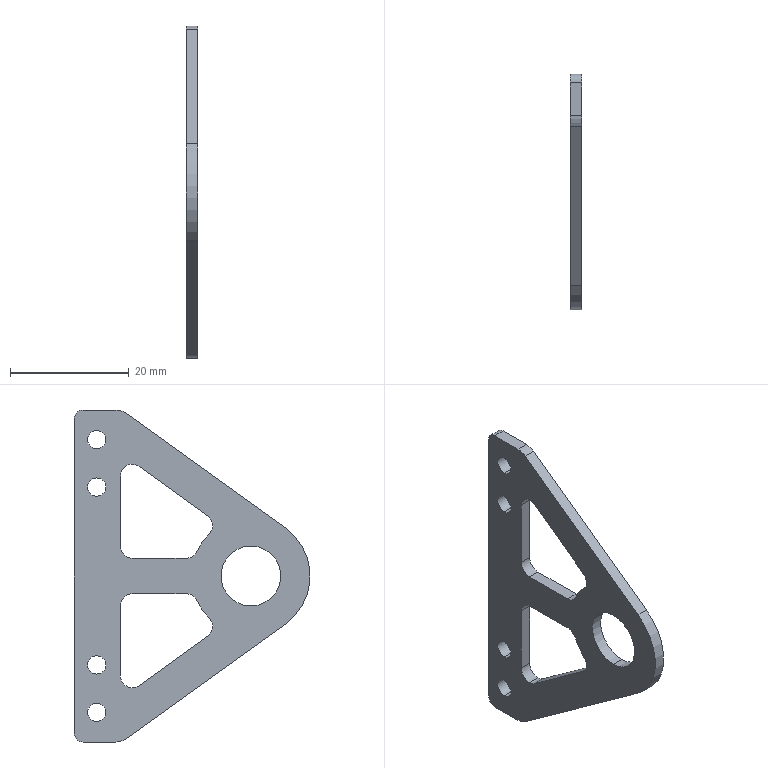Part | SolidWorks | features Fillet 4, Extrusion 1, ICE 1, MirrorPattern 1 | 1 solid | 39 faces | box 2 x 39.8 x 56 mm | volume 2062 mm3 | cylinder 26 | plane 13 | commonest cylinder face diameters 4 x9 3.1 x8 20 x3 3 x2 6 x2 10.1 x2
STEP:
#1=CARTESIAN_POINT('',(0.,20.,-18.85));
#2=VERTEX_POINT('',#1);
#3=CARTESIAN_POINT('',(0.,22.,-16.85));
#4=VERTEX_POINT('',#3);
#5=CARTESIAN_POINT('',(0.,20.,-16.85));
#6=DIRECTION('',(1.,0.,0.));
#7=DIRECTION('',(0.,0.,-1.));
#8=AXIS2_PLACEMENT_3D('',#5,#6,#7);
#9=CIRCLE('',#8,2.);
#10=EDGE_CURVE('',#2,#4,#9,.T.);
#11=ORIENTED_EDGE('',*,*,#10,.F.);
#12=CARTESIAN_POINT('',(2.,20.,-18.85));
#13=VERTEX_POINT('',#12);
#14=CARTESIAN_POINT('',(2.,20.,-18.85));
#15=DIRECTION('',(1.,0.,0.));
#16=VECTOR('',#15,1000.);
#17=LINE('',#14,#16);
#18=EDGE_CURVE('',#2,#13,#17,.T.);
#19=ORIENTED_EDGE('',*,*,#18,.T.);
#20=CARTESIAN_POINT('',(2.,22.,-16.85));
#21=VERTEX_POINT('',#20);
#22=CARTESIAN_POINT('',(2.,20.,-16.85));
#23=DIRECTION('',(-1.,0.,0.));
#24=DIRECTION('',(0.,0.,-1.));
#25=AXIS2_PLACEMENT_3D('',#22,#23,#24);
#26=CIRCLE('',#25,2.);
#27=EDGE_CURVE('',#21,#13,#26,.T.);
#28=ORIENTED_EDGE('',*,*,#27,.F.);
#29=CARTESIAN_POINT('',(2.,22.,-16.85));
#30=DIRECTION('',(1.,0.,0.));
#31=VECTOR('',#30,1000.);
#32=LINE('',#29,#31);
#33=EDGE_CURVE('',#4,#21,#32,.T.);
#34=ORIENTED_EDGE('',*,*,#33,.F.);
#35=EDGE_LOOP('',(#11,#19,#28,#34));
#36=FACE_OUTER_BOUND('',#35,.T.);
#37=CARTESIAN_POINT('',(2.,20.,-16.85));
#38=DIRECTION('',(1.,0.,0.));
#39=DIRECTION('',(0.,0.,-1.));
#40=AXIS2_PLACEMENT_3D('',#37,#38,#39);
#41=CYLINDRICAL_SURFACE('',#40,2.);
#42=ADVANCED_FACE('',(#36),#41,.F.);
#43=CARTESIAN_POINT('',(2.,26.,-13.45));
#44=VERTEX_POINT('',#43);
#45=CARTESIAN_POINT('',(2.,26.,-16.55));
#46=VERTEX_POINT('',#45);
#47=CARTESIAN_POINT('',(2.,26.,-15.));
#48=DIRECTION('',(1.,0.,0.));
#49=DIRECTION('',(0.,0.,1.));
#50=AXIS2_PLACEMENT_3D('',#47,#48,#49);
#51=CIRCLE('',#50,1.55);
#52=EDGE_CURVE('',#44,#46,#51,.T.);
#53=ORIENTED_EDGE('',*,*,#52,.T.);
#54=CARTESIAN_POINT('',(0.,26.,-16.55));
#55=VERTEX_POINT('',#54);
#56=CARTESIAN_POINT('',(2.,26.,-16.55));
#57=DIRECTION('',(-1.,0.,0.));
#58=VECTOR('',#57,1000.);
#59=LINE('',#56,#58);
#60=EDGE_CURVE('',#46,#55,#59,.T.);
#61=ORIENTED_EDGE('',*,*,#60,.T.);
#62=CARTESIAN_POINT('',(0.,26.,-13.45));
#63=VERTEX_POINT('',#62);
#64=CARTESIAN_POINT('',(0.,26.,-15.));
#65=DIRECTION('',(1.,0.,0.));
#66=DIRECTION('',(0.,0.,1.));
#67=AXIS2_PLACEMENT_3D('',#64,#65,#66);
#68=CIRCLE('',#67,1.55);
#69=EDGE_CURVE('',#63,#55,#68,.T.);
#70=ORIENTED_EDGE('',*,*,#69,.F.);
#71=CARTESIAN_POINT('',(2.,26.,-13.45));
#72=DIRECTION('',(-1.,0.,0.));
#73=VECTOR('',#72,1000.);
#74=LINE('',#71,#73);
#75=EDGE_CURVE('',#44,#63,#74,.T.);
#76=ORIENTED_EDGE('',*,*,#75,.F.);
#77=EDGE_LOOP('',(#53,#61,#70,#76));
#78=FACE_OUTER_BOUND('',#77,.T.);
#79=CARTESIAN_POINT('',(2.,26.,-15.));
#80=DIRECTION('',(-1.,0.,0.));
#81=DIRECTION('',(0.,0.,1.));
#82=AXIS2_PLACEMENT_3D('',#79,#80,#81);
#83=CYLINDRICAL_SURFACE('',#82,1.55);
#84=ADVANCED_FACE('',(#78),#83,.F.);
#85=CARTESIAN_POINT('',(2.,26.,-21.45));
#86=VERTEX_POINT('',#85);
#87=CARTESIAN_POINT('',(2.,26.,-24.55));
#88=VERTEX_POINT('',#87);
#89=CARTESIAN_POINT('',(2.,26.,-23.));
#90=DIRECTION('',(1.,0.,0.));
#91=DIRECTION('',(0.,0.,1.));
#92=AXIS2_PLACEMENT_3D('',#89,#90,#91);
#93=CIRCLE('',#92,1.55);
#94=EDGE_CURVE('',#86,#88,#93,.T.);
#95=ORIENTED_EDGE('',*,*,#94,.T.);
#96=CARTESIAN_POINT('',(0.,26.,-24.55));
#97=VERTEX_POINT('',#96);
#98=CARTESIAN_POINT('',(2.,26.,-24.55));
#99=DIRECTION('',(-1.,0.,0.));
#100=VECTOR('',#99,1000.);
#101=LINE('',#98,#100);
#102=EDGE_CURVE('',#88,#97,#101,.T.);
#103=ORIENTED_EDGE('',*,*,#102,.T.);
#104=CARTESIAN_POINT('',(0.,26.,-21.45));
#105=VERTEX_POINT('',#104);
#106=CARTESIAN_POINT('',(0.,26.,-23.));
#107=DIRECTION('',(1.,0.,0.));
#108=DIRECTION('',(0.,0.,1.));
#109=AXIS2_PLACEMENT_3D('',#106,#107,#108);
#110=CIRCLE('',#109,1.55);
#111=EDGE_CURVE('',#105,#97,#110,.T.);
#112=ORIENTED_EDGE('',*,*,#111,.F.);
#113=CARTESIAN_POINT('',(2.,26.,-21.45));
#114=DIRECTION('',(-1.,0.,0.));
#115=VECTOR('',#114,1000.);
#116=LINE('',#113,#115);
#117=EDGE_CURVE('',#86,#105,#116,.T.);
#118=ORIENTED_EDGE('',*,*,#117,.F.);
#119=EDGE_LOOP('',(#95,#103,#112,#118));
#120=FACE_OUTER_BOUND('',#119,.T.);
#121=CARTESIAN_POINT('',(2.,26.,-23.));
#122=DIRECTION('',(-1.,0.,0.));
#123=DIRECTION('',(0.,0.,1.));
#124=AXIS2_PLACEMENT_3D('',#121,#122,#123);
#125=CYLINDRICAL_SURFACE('',#124,1.55);
#126=ADVANCED_FACE('',(#120),#125,.F.);
#127=CARTESIAN_POINT('',(2.,26.,24.55));
#128=VERTEX_POINT('',#127);
#129=CARTESIAN_POINT('',(2.,26.,21.45));
#130=VERTEX_POINT('',#129);
#131=CARTESIAN_POINT('',(2.,26.,23.));
#132=DIRECTION('',(1.,0.,0.));
#133=DIRECTION('',(0.,0.,-1.));
#134=AXIS2_PLACEMENT_3D('',#131,#132,#133);
#135=CIRCLE('',#134,1.55);
#136=EDGE_CURVE('',#128,#130,#135,.T.);
#137=ORIENTED_EDGE('',*,*,#136,.T.);
#138=CARTESIAN_POINT('',(0.,26.,21.45));
#139=VERTEX_POINT('',#138);
#140=CARTESIAN_POINT('',(2.,26.,21.45));
#141=DIRECTION('',(-1.,0.,0.));
#142=VECTOR('',#141,1000.);
#143=LINE('',#140,#142);
#144=EDGE_CURVE('',#130,#139,#143,.T.);
#145=ORIENTED_EDGE('',*,*,#144,.T.);
#146=CARTESIAN_POINT('',(0.,26.,24.55));
#147=VERTEX_POINT('',#146);
#148=CARTESIAN_POINT('',(0.,26.,23.));
#149=DIRECTION('',(1.,0.,0.));
#150=DIRECTION('',(0.,0.,-1.));
#151=AXIS2_PLACEMENT_3D('',#148,#149,#150);
#152=CIRCLE('',#151,1.55);
#153=EDGE_CURVE('',#147,#139,#152,.T.);
#154=ORIENTED_EDGE('',*,*,#153,.F.);
#155=CARTESIAN_POINT('',(2.,26.,24.55));
#156=DIRECTION('',(-1.,0.,0.));
#157=VECTOR('',#156,1000.);
#158=LINE('',#155,#157);
#159=EDGE_CURVE('',#128,#147,#158,.T.);
#160=ORIENTED_EDGE('',*,*,#159,.F.);
#161=EDGE_LOOP('',(#137,#145,#154,#160));
#162=FACE_OUTER_BOUND('',#161,.T.);
#163=CARTESIAN_POINT('',(2.,26.,23.));
#164=DIRECTION('',(-1.,0.,0.));
#165=DIRECTION('',(0.,0.,1.));
#166=AXIS2_PLACEMENT_3D('',#163,#164,#165);
#167=CYLINDRICAL_SURFACE('',#166,1.55);
#168=ADVANCED_FACE('',(#162),#167,.F.);
#169=CARTESIAN_POINT('',(2.,26.,16.55));
#170=VERTEX_POINT('',#169);
#171=CARTESIAN_POINT('',(2.,26.,13.45));
#172=VERTEX_POINT('',#171);
#173=CARTESIAN_POINT('',(2.,26.,15.));
#174=DIRECTION('',(1.,0.,0.));
#175=DIRECTION('',(0.,0.,-1.));
#176=AXIS2_PLACEMENT_3D('',#173,#174,#175);
#177=CIRCLE('',#176,1.55);
#178=EDGE_CURVE('',#170,#172,#177,.T.);
#179=ORIENTED_EDGE('',*,*,#178,.T.);
#180=CARTESIAN_POINT('',(0.,26.,13.45));
#181=VERTEX_POINT('',#180);
#182=CARTESIAN_POINT('',(2.,26.,13.45));
#183=DIRECTION('',(-1.,0.,0.));
#184=VECTOR('',#183,1000.);
#185=LINE('',#182,#184);
#186=EDGE_CURVE('',#172,#181,#185,.T.);
#187=ORIENTED_EDGE('',*,*,#186,.T.);
#188=CARTESIAN_POINT('',(0.,26.,16.55));
#189=VERTEX_POINT('',#188);
#190=CARTESIAN_POINT('',(0.,26.,15.));
#191=DIRECTION('',(1.,0.,0.));
#192=DIRECTION('',(0.,0.,-1.));
#193=AXIS2_PLACEMENT_3D('',#190,#191,#192);
#194=CIRCLE('',#193,1.55);
#195=EDGE_CURVE('',#189,#181,#194,.T.);
#196=ORIENTED_EDGE('',*,*,#195,.F.);
#197=CARTESIAN_POINT('',(2.,26.,16.55));
#198=DIRECTION('',(-1.,0.,0.));
#199=VECTOR('',#198,1000.);
#200=LINE('',#197,#199);
#201=EDGE_CURVE('',#170,#189,#200,.T.);
#202=ORIENTED_EDGE('',*,*,#201,.F.);
#203=EDGE_LOOP('',(#179,#187,#196,#202));
#204=FACE_OUTER_BOUND('',#203,.T.);
#205=CARTESIAN_POINT('',(2.,26.,15.));
#206=DIRECTION('',(-1.,0.,0.));
#207=DIRECTION('',(0.,0.,1.));
#208=AXIS2_PLACEMENT_3D('',#205,#206,#207);
#209=CYLINDRICAL_SURFACE('',#208,1.55);
#210=ADVANCED_FACE('',(#204),#209,.F.);
#211=CARTESIAN_POINT('',(2.,0.,5.05));
#212=VERTEX_POINT('',#211);
#213=CARTESIAN_POINT('',(2.,0.,-5.05));
#214=VERTEX_POINT('',#213);
#215=CARTESIAN_POINT('',(2.,0.,0.));
#216=DIRECTION('',(1.,0.,0.));
#217=DIRECTION('',(0.,0.,-1.));
#218=AXIS2_PLACEMENT_3D('',#215,#216,#217);
#219=CIRCLE('',#218,5.05);
#220=EDGE_CURVE('',#212,#214,#219,.T.);
#221=ORIENTED_EDGE('',*,*,#220,.T.);
#222=CARTESIAN_POINT('',(0.,0.,-5.05));
#223=VERTEX_POINT('',#222);
#224=CARTESIAN_POINT('',(2.,0.,-5.05));
#225=DIRECTION('',(-1.,0.,0.));
#226=VECTOR('',#225,1000.);
#227=LINE('',#224,#226);
#228=EDGE_CURVE('',#214,#223,#227,.T.);
#229=ORIENTED_EDGE('',*,*,#228,.T.);
#230=CARTESIAN_POINT('',(0.,0.,5.05));
#231=VERTEX_POINT('',#230);
#232=CARTESIAN_POINT('',(0.,0.,0.));
#233=DIRECTION('',(1.,0.,0.));
#234=DIRECTION('',(0.,0.,-1.));
#235=AXIS2_PLACEMENT_3D('',#232,#233,#234);
#236=CIRCLE('',#235,5.05);
#237=EDGE_CURVE('',#231,#223,#236,.T.);
#238=ORIENTED_EDGE('',*,*,#237,.F.);
#239=CARTESIAN_POINT('',(2.,0.,5.05));
#240=DIRECTION('',(-1.,0.,0.));
#241=VECTOR('',#240,1000.);
#242=LINE('',#239,#241);
#243=EDGE_CURVE('',#212,#231,#242,.T.);
#244=ORIENTED_EDGE('',*,*,#243,.F.);
#245=EDGE_LOOP('',(#221,#229,#238,#244));
#246=FACE_OUTER_BOUND('',#245,.T.);
#247=CARTESIAN_POINT('',(2.,0.,0.));
#248=DIRECTION('',(-1.,0.,0.));
#249=DIRECTION('',(0.,0.,1.));
#250=AXIS2_PLACEMENT_3D('',#247,#248,#249);
#251=CYLINDRICAL_SURFACE('',#250,5.05);
#252=ADVANCED_FACE('',(#246),#251,.F.);
#253=CARTESIAN_POINT('',(2.,10.909,-3.));
#254=VERTEX_POINT('',#253);
#255=CARTESIAN_POINT('',(2.,20.,-3.));
#256=VERTEX_POINT('',#255);
#257=CARTESIAN_POINT('',(2.,22.,-3.));
#258=DIRECTION('',(0.,1.,0.));
#259=VECTOR('',#258,1000.);
#260=LINE('',#257,#259);
#261=EDGE_CURVE('',#254,#256,#260,.T.);
#262=ORIENTED_EDGE('',*,*,#261,.T.);
#263=CARTESIAN_POINT('',(2.,22.,-5.));
#264=VERTEX_POINT('',#263);
#265=CARTESIAN_POINT('',(2.,20.,-5.));
#266=DIRECTION('',(-1.,0.,0.));
#267=DIRECTION('',(0.,0.,-1.));
#268=AXIS2_PLACEMENT_3D('',#265,#266,#267);
#269=CIRCLE('',#268,2.);
#270=EDGE_CURVE('',#256,#264,#269,.T.);
#271=ORIENTED_EDGE('',*,*,#270,.T.);
#272=CARTESIAN_POINT('',(2.,22.,-20.753));
#273=DIRECTION('',(0.,0.,-1.));
#274=VECTOR('',#273,1000.);
#275=LINE('',#272,#274);
#276=EDGE_CURVE('',#264,#21,#275,.T.);
#277=ORIENTED_EDGE('',*,*,#276,.T.);
#278=ORIENTED_EDGE('',*,*,#27,.T.);
#279=CARTESIAN_POINT('',(2.,18.832,-18.474));
#280=VERTEX_POINT('',#279);
#281=CARTESIAN_POINT('',(2.,20.,-16.85));
#282=DIRECTION('',(-1.,0.,0.));
#283=DIRECTION('',(0.,0.,-1.));
#284=AXIS2_PLACEMENT_3D('',#281,#282,#283);
#285=CIRCLE('',#284,2.);
#286=EDGE_CURVE('',#13,#280,#285,.T.);
#287=ORIENTED_EDGE('',*,*,#286,.T.);
#288=CARTESIAN_POINT('',(2.,7.269,-10.157));
#289=VERTEX_POINT('',#288);
#290=CARTESIAN_POINT('',(2.,22.,-20.753));
#291=DIRECTION('',(0.,-0.8118,0.5839));
#292=VECTOR('',#291,1000.);
#293=LINE('',#290,#292);
#294=EDGE_CURVE('',#280,#289,#293,.T.);
#295=ORIENTED_EDGE('',*,*,#294,.T.);
#296=CARTESIAN_POINT('',(2.,7.031,-7.111));
#297=VERTEX_POINT('',#296);
#298=CARTESIAN_POINT('',(2.,8.437,-8.533));
#299=DIRECTION('',(-1.,0.,0.));
#300=DIRECTION('',(0.,0.,-1.));
#301=AXIS2_PLACEMENT_3D('',#298,#299,#300);
#302=CIRCLE('',#301,2.);
#303=EDGE_CURVE('',#289,#297,#302,.T.);
#304=ORIENTED_EDGE('',*,*,#303,.T.);
#305=CARTESIAN_POINT('',(2.,9.091,-4.167));
#306=VERTEX_POINT('',#305);
#307=CARTESIAN_POINT('',(2.,0.,0.));
#308=DIRECTION('',(1.,0.,0.));
#309=DIRECTION('',(0.,0.,1.));
#310=AXIS2_PLACEMENT_3D('',#307,#308,#309);
#311=CIRCLE('',#310,10.);
#312=EDGE_CURVE('',#297,#306,#311,.T.);
#313=ORIENTED_EDGE('',*,*,#312,.T.);
#314=CARTESIAN_POINT('',(2.,10.909,-5.));
#315=DIRECTION('',(-1.,0.,0.));
#316=DIRECTION('',(0.,0.,-1.));
#317=AXIS2_PLACEMENT_3D('',#314,#315,#316);
#318=CIRCLE('',#317,2.);
#319=EDGE_CURVE('',#306,#254,#318,.T.);
#320=ORIENTED_EDGE('',*,*,#319,.T.);
#321=EDGE_LOOP('',(#262,#271,#277,#278,#287,#295,#304,#313,#320));
#322=FACE_BOUND('',#321,.T.);
#323=ORIENTED_EDGE('',*,*,#94,.F.);
#324=CARTESIAN_POINT('',(2.,26.,-23.));
#325=DIRECTION('',(1.,0.,0.));
#326=DIRECTION('',(0.,0.,1.));
#327=AXIS2_PLACEMENT_3D('',#324,#325,#326);
#328=CIRCLE('',#327,1.55);
#329=EDGE_CURVE('',#88,#86,#328,.T.);
#330=ORIENTED_EDGE('',*,*,#329,.F.);
#331=EDGE_LOOP('',(#323,#330));
#332=FACE_BOUND('',#331,.T.);
#333=ORIENTED_EDGE('',*,*,#178,.F.);
#334=CARTESIAN_POINT('',(2.,26.,15.));
#335=DIRECTION('',(1.,0.,0.));
#336=DIRECTION('',(0.,0.,-1.));
#337=AXIS2_PLACEMENT_3D('',#334,#335,#336);
#338=CIRCLE('',#337,1.55);
#339=EDGE_CURVE('',#172,#170,#338,.T.);
#340=ORIENTED_EDGE('',*,*,#339,.F.);
#341=EDGE_LOOP('',(#333,#340));
#342=FACE_BOUND('',#341,.T.);
#343=CARTESIAN_POINT('',(2.,22.767,-28.));
#344=VERTEX_POINT('',#343);
#345=CARTESIAN_POINT('',(2.,28.3,-28.));
#346=VERTEX_POINT('',#345);
#347=CARTESIAN_POINT('',(2.,29.8,-28.));
#348=DIRECTION('',(0.,1.,0.));
#349=VECTOR('',#348,1000.);
#350=LINE('',#347,#349);
#351=EDGE_CURVE('',#344,#346,#350,.T.);
#352=ORIENTED_EDGE('',*,*,#351,.T.);
#353=CARTESIAN_POINT('',(2.,29.8,-26.5));
#354=VERTEX_POINT('',#353);
#355=CARTESIAN_POINT('',(2.,28.3,-26.5));
#356=DIRECTION('',(1.,0.,0.));
#357=DIRECTION('',(0.,0.,-1.));
#358=AXIS2_PLACEMENT_3D('',#355,#356,#357);
#359=CIRCLE('',#358,1.5);
#360=EDGE_CURVE('',#346,#354,#359,.T.);
#361=ORIENTED_EDGE('',*,*,#360,.T.);
#362=CARTESIAN_POINT('',(2.,29.8,26.5));
#363=VERTEX_POINT('',#362);
#364=CARTESIAN_POINT('',(2.,29.8,-28.));
#365=DIRECTION('',(0.,0.,1.));
#366=VECTOR('',#365,1000.);
#367=LINE('',#364,#366);
#368=EDGE_CURVE('',#354,#363,#367,.T.);
#369=ORIENTED_EDGE('',*,*,#368,.T.);
#370=CARTESIAN_POINT('',(2.,28.3,28.));
#371=VERTEX_POINT('',#370);
#372=CARTESIAN_POINT('',(2.,28.3,26.5));
#373=DIRECTION('',(1.,0.,0.));
#374=DIRECTION('',(0.,0.,-1.));
#375=AXIS2_PLACEMENT_3D('',#372,#373,#374);
#376=CIRCLE('',#375,1.5);
#377=EDGE_CURVE('',#363,#371,#376,.T.);
#378=ORIENTED_EDGE('',*,*,#377,.T.);
#379=CARTESIAN_POINT('',(2.,22.767,28.));
#380=VERTEX_POINT('',#379);
#381=CARTESIAN_POINT('',(2.,29.8,28.));
#382=DIRECTION('',(0.,-1.,0.));
#383=VECTOR('',#382,1000.);
#384=LINE('',#381,#383);
#385=EDGE_CURVE('',#371,#380,#384,.T.);
#386=ORIENTED_EDGE('',*,*,#385,.T.);
#387=CARTESIAN_POINT('',(2.,21.015,27.435));
#388=VERTEX_POINT('',#387);
#389=CARTESIAN_POINT('',(2.,22.767,25.));
#390=DIRECTION('',(1.,0.,0.));
#391=DIRECTION('',(0.,0.,-1.));
#392=AXIS2_PLACEMENT_3D('',#389,#390,#391);
#393=CIRCLE('',#392,3.);
#394=EDGE_CURVE('',#380,#388,#393,.T.);
#395=ORIENTED_EDGE('',*,*,#394,.T.);
#396=CARTESIAN_POINT('',(2.,-5.839,8.118));
#397=VERTEX_POINT('',#396);
#398=CARTESIAN_POINT('',(2.,21.8,28.));
#399=DIRECTION('',(0.,-0.8118,-0.5839));
#400=VECTOR('',#399,1000.);
#401=LINE('',#398,#400);
#402=EDGE_CURVE('',#388,#397,#401,.T.);
#403=ORIENTED_EDGE('',*,*,#402,.T.);
#404=CARTESIAN_POINT('',(2.,-5.839,-8.118));
#405=VERTEX_POINT('',#404);
#406=CARTESIAN_POINT('',(2.,0.,0.));
#407=DIRECTION('',(1.,0.,0.));
#408=DIRECTION('',(0.,0.,-1.));
#409=AXIS2_PLACEMENT_3D('',#406,#407,#408);
#410=CIRCLE('',#409,10.);
#411=EDGE_CURVE('',#397,#405,#410,.T.);
#412=ORIENTED_EDGE('',*,*,#411,.T.);
#413=CARTESIAN_POINT('',(2.,21.015,-27.435));
#414=VERTEX_POINT('',#413);
#415=CARTESIAN_POINT('',(2.,21.8,-28.));
#416=DIRECTION('',(0.,0.8118,-0.5839));
#417=VECTOR('',#416,1000.);
#418=LINE('',#415,#417);
#419=EDGE_CURVE('',#405,#414,#418,.T.);
#420=ORIENTED_EDGE('',*,*,#419,.T.);
#421=CARTESIAN_POINT('',(2.,22.767,-25.));
#422=DIRECTION('',(1.,0.,0.));
#423=DIRECTION('',(0.,0.,-1.));
#424=AXIS2_PLACEMENT_3D('',#421,#422,#423);
#425=CIRCLE('',#424,3.);
#426=EDGE_CURVE('',#414,#344,#425,.T.);
#427=ORIENTED_EDGE('',*,*,#426,.T.);
#428=EDGE_LOOP('',(#352,#361,#369,#378,#386,#395,#403,#412,#420,#427));
#429=FACE_OUTER_BOUND('',#428,.T.);
#430=ORIENTED_EDGE('',*,*,#220,.F.);
#431=CARTESIAN_POINT('',(2.,0.,0.));
#432=DIRECTION('',(1.,0.,0.));
#433=DIRECTION('',(0.,0.,-1.));
#434=AXIS2_PLACEMENT_3D('',#431,#432,#433);
#435=CIRCLE('',#434,5.05);
#436=EDGE_CURVE('',#214,#212,#435,.T.);
#437=ORIENTED_EDGE('',*,*,#436,.F.);
#438=EDGE_LOOP('',(#430,#437));
#439=FACE_BOUND('',#438,.T.);
#440=ORIENTED_EDGE('',*,*,#136,.F.);
#441=CARTESIAN_POINT('',(2.,26.,23.));
#442=DIRECTION('',(1.,0.,0.));
#443=DIRECTION('',(0.,0.,-1.));
#444=AXIS2_PLACEMENT_3D('',#441,#442,#443);
#445=CIRCLE('',#444,1.55);
#446=EDGE_CURVE('',#130,#128,#445,.T.);
#447=ORIENTED_EDGE('',*,*,#446,.F.);
#448=EDGE_LOOP('',(#440,#447));
#449=FACE_BOUND('',#448,.T.);
#450=ORIENTED_EDGE('',*,*,#52,.F.);
#451=CARTESIAN_POINT('',(2.,26.,-15.));
#452=DIRECTION('',(1.,0.,0.));
#453=DIRECTION('',(0.,0.,1.));
#454=AXIS2_PLACEMENT_3D('',#451,#452,#453);
#455=CIRCLE('',#454,1.55);
#456=EDGE_CURVE('',#46,#44,#455,.T.);
#457=ORIENTED_EDGE('',*,*,#456,.F.);
#458=EDGE_LOOP('',(#450,#457));
#459=FACE_BOUND('',#458,.T.);
#460=CARTESIAN_POINT('',(2.,18.832,18.474));
#461=VERTEX_POINT('',#460);
#462=CARTESIAN_POINT('',(2.,7.269,10.157));
#463=VERTEX_POINT('',#462);
#464=CARTESIAN_POINT('',(2.,22.,20.753));
#465=DIRECTION('',(0.,-0.8118,-0.5839));
#466=VECTOR('',#465,1000.);
#467=LINE('',#464,#466);
#468=EDGE_CURVE('',#461,#463,#467,.T.);
#469=ORIENTED_EDGE('',*,*,#468,.F.);
#470=CARTESIAN_POINT('',(2.,22.,16.85));
#471=VERTEX_POINT('',#470);
#472=CARTESIAN_POINT('',(2.,20.,16.85));
#473=DIRECTION('',(-1.,0.,0.));
#474=DIRECTION('',(0.,0.,-1.));
#475=AXIS2_PLACEMENT_3D('',#472,#473,#474);
#476=CIRCLE('',#475,2.);
#477=EDGE_CURVE('',#461,#471,#476,.T.);
#478=ORIENTED_EDGE('',*,*,#477,.T.);
#479=CARTESIAN_POINT('',(2.,22.,5.));
#480=VERTEX_POINT('',#479);
#481=CARTESIAN_POINT('',(2.,22.,20.753));
#482=DIRECTION('',(0.,0.,1.));
#483=VECTOR('',#482,1000.);
#484=LINE('',#481,#483);
#485=EDGE_CURVE('',#480,#471,#484,.T.);
#486=ORIENTED_EDGE('',*,*,#485,.F.);
#487=CARTESIAN_POINT('',(2.,20.,3.));
#488=VERTEX_POINT('',#487);
#489=CARTESIAN_POINT('',(2.,20.,5.));
#490=DIRECTION('',(-1.,0.,0.));
#491=DIRECTION('',(0.,0.,-1.));
#492=AXIS2_PLACEMENT_3D('',#489,#490,#491);
#493=CIRCLE('',#492,2.);
#494=EDGE_CURVE('',#480,#488,#493,.T.);
#495=ORIENTED_EDGE('',*,*,#494,.T.);
#496=CARTESIAN_POINT('',(2.,10.909,3.));
#497=VERTEX_POINT('',#496);
#498=CARTESIAN_POINT('',(2.,22.,3.));
#499=DIRECTION('',(0.,1.,0.));
#500=VECTOR('',#499,1000.);
#501=LINE('',#498,#500);
#502=EDGE_CURVE('',#497,#488,#501,.T.);
#503=ORIENTED_EDGE('',*,*,#502,.F.);
#504=CARTESIAN_POINT('',(2.,9.091,4.167));
#505=VERTEX_POINT('',#504);
#506=CARTESIAN_POINT('',(2.,10.909,5.));
#507=DIRECTION('',(-1.,0.,0.));
#508=DIRECTION('',(0.,0.,-1.));
#509=AXIS2_PLACEMENT_3D('',#506,#507,#508);
#510=CIRCLE('',#509,2.);
#511=EDGE_CURVE('',#497,#505,#510,.T.);
#512=ORIENTED_EDGE('',*,*,#511,.T.);
#513=CARTESIAN_POINT('',(2.,7.031,7.111));
#514=VERTEX_POINT('',#513);
#515=CARTESIAN_POINT('',(2.,0.,0.));
#516=DIRECTION('',(-1.,0.,0.));
#517=DIRECTION('',(0.,0.,-1.));
#518=AXIS2_PLACEMENT_3D('',#515,#516,#517);
#519=CIRCLE('',#518,10.);
#520=EDGE_CURVE('',#514,#505,#519,.T.);
#521=ORIENTED_EDGE('',*,*,#520,.F.);
#522=CARTESIAN_POINT('',(2.,8.437,8.533));
#523=DIRECTION('',(-1.,0.,0.));
#524=DIRECTION('',(0.,0.,-1.));
#525=AXIS2_PLACEMENT_3D('',#522,#523,#524);
#526=CIRCLE('',#525,2.);
#527=EDGE_CURVE('',#514,#463,#526,.T.);
#528=ORIENTED_EDGE('',*,*,#527,.T.);
#529=EDGE_LOOP('',(#469,#478,#486,#495,#503,#512,#521,#528));
#530=FACE_BOUND('',#529,.T.);
#531=CARTESIAN_POINT('',(2.,0.,0.));
#532=DIRECTION('',(1.,0.,0.));
#533=DIRECTION('',(0.,0.,-1.));
#534=AXIS2_PLACEMENT_3D('',#531,#532,#533);
#535=PLANE('',#534);
#536=ADVANCED_FACE('',(#322,#332,#342,#429,#439,#449,#459,#530),#535,.T.);
#537=CARTESIAN_POINT('',(0.,18.832,-18.474));
#538=VERTEX_POINT('',#537);
#539=CARTESIAN_POINT('',(0.,7.269,-10.157));
#540=VERTEX_POINT('',#539);
#541=CARTESIAN_POINT('',(0.,22.,-20.753));
#542=DIRECTION('',(0.,-0.8118,0.5839));
#543=VECTOR('',#542,1000.);
#544=LINE('',#541,#543);
#545=EDGE_CURVE('',#538,#540,#544,.T.);
#546=ORIENTED_EDGE('',*,*,#545,.F.);
#547=CARTESIAN_POINT('',(0.,20.,-16.85));
#548=DIRECTION('',(1.,0.,0.));
#549=DIRECTION('',(0.,0.,-1.));
#550=AXIS2_PLACEMENT_3D('',#547,#548,#549);
#551=CIRCLE('',#550,2.);
#552=EDGE_CURVE('',#538,#2,#551,.T.);
#553=ORIENTED_EDGE('',*,*,#552,.T.);
#554=ORIENTED_EDGE('',*,*,#10,.T.);
#555=CARTESIAN_POINT('',(0.,22.,-5.));
#556=VERTEX_POINT('',#555);
#557=CARTESIAN_POINT('',(0.,22.,-20.753));
#558=DIRECTION('',(0.,0.,-1.));
#559=VECTOR('',#558,1000.);
#560=LINE('',#557,#559);
#561=EDGE_CURVE('',#556,#4,#560,.T.);
#562=ORIENTED_EDGE('',*,*,#561,.F.);
#563=CARTESIAN_POINT('',(0.,20.,-3.));
#564=VERTEX_POINT('',#563);
#565=CARTESIAN_POINT('',(0.,20.,-5.));
#566=DIRECTION('',(1.,0.,0.));
#567=DIRECTION('',(0.,0.,-1.));
#568=AXIS2_PLACEMENT_3D('',#565,#566,#567);
#569=CIRCLE('',#568,2.);
#570=EDGE_CURVE('',#556,#564,#569,.T.);
#571=ORIENTED_EDGE('',*,*,#570,.T.);
#572=CARTESIAN_POINT('',(0.,10.909,-3.));
#573=VERTEX_POINT('',#572);
#574=CARTESIAN_POINT('',(0.,22.,-3.));
#575=DIRECTION('',(0.,1.,0.));
#576=VECTOR('',#575,1000.);
#577=LINE('',#574,#576);
#578=EDGE_CURVE('',#573,#564,#577,.T.);
#579=ORIENTED_EDGE('',*,*,#578,.F.);
#580=CARTESIAN_POINT('',(0.,9.091,-4.167));
#581=VERTEX_POINT('',#580);
#582=CARTESIAN_POINT('',(0.,10.909,-5.));
#583=DIRECTION('',(1.,0.,0.));
#584=DIRECTION('',(0.,0.,-1.));
#585=AXIS2_PLACEMENT_3D('',#582,#583,#584);
#586=CIRCLE('',#585,2.);
#587=EDGE_CURVE('',#573,#581,#586,.T.);
#588=ORIENTED_EDGE('',*,*,#587,.T.);
#589=CARTESIAN_POINT('',(0.,7.031,-7.111));
#590=VERTEX_POINT('',#589);
#591=CARTESIAN_POINT('',(0.,0.,0.));
#592=DIRECTION('',(1.,0.,0.));
#593=DIRECTION('',(0.,0.,1.));
#594=AXIS2_PLACEMENT_3D('',#591,#592,#593);
#595=CIRCLE('',#594,10.);
#596=EDGE_CURVE('',#590,#581,#595,.T.);
#597=ORIENTED_EDGE('',*,*,#596,.F.);
#598=CARTESIAN_POINT('',(0.,8.437,-8.533));
#599=DIRECTION('',(1.,0.,0.));
#600=DIRECTION('',(0.,0.,-1.));
#601=AXIS2_PLACEMENT_3D('',#598,#599,#600);
#602=CIRCLE('',#601,2.);
#603=EDGE_CURVE('',#590,#540,#602,.T.);
#604=ORIENTED_EDGE('',*,*,#603,.T.);
#605=EDGE_LOOP('',(#546,#553,#554,#562,#571,#579,#588,#597,#604));
#606=FACE_BOUND('',#605,.T.);
#607=ORIENTED_EDGE('',*,*,#69,.T.);
#608=CARTESIAN_POINT('',(0.,26.,-15.));
#609=DIRECTION('',(1.,0.,0.));
#610=DIRECTION('',(0.,0.,1.));
#611=AXIS2_PLACEMENT_3D('',#608,#609,#610);
#612=CIRCLE('',#611,1.55);
#613=EDGE_CURVE('',#55,#63,#612,.T.);
#614=ORIENTED_EDGE('',*,*,#613,.T.);
#615=EDGE_LOOP('',(#607,#614));
#616=FACE_BOUND('',#615,.T.);
#617=ORIENTED_EDGE('',*,*,#111,.T.);
#618=CARTESIAN_POINT('',(0.,26.,-23.));
#619=DIRECTION('',(1.,0.,0.));
#620=DIRECTION('',(0.,0.,1.));
#621=AXIS2_PLACEMENT_3D('',#618,#619,#620);
#622=CIRCLE('',#621,1.55);
#623=EDGE_CURVE('',#97,#105,#622,.T.);
#624=ORIENTED_EDGE('',*,*,#623,.T.);
#625=EDGE_LOOP('',(#617,#624));
#626=FACE_BOUND('',#625,.T.);
#627=ORIENTED_EDGE('',*,*,#153,.T.);
#628=CARTESIAN_POINT('',(0.,26.,23.));
#629=DIRECTION('',(1.,0.,0.));
#630=DIRECTION('',(0.,0.,-1.));
#631=AXIS2_PLACEMENT_3D('',#628,#629,#630);
#632=CIRCLE('',#631,1.55);
#633=EDGE_CURVE('',#139,#147,#632,.T.);
#634=ORIENTED_EDGE('',*,*,#633,.T.);
#635=EDGE_LOOP('',(#627,#634));
#636=FACE_BOUND('',#635,.T.);
#637=ORIENTED_EDGE('',*,*,#195,.T.);
#638=CARTESIAN_POINT('',(0.,26.,15.));
#639=DIRECTION('',(1.,0.,0.));
#640=DIRECTION('',(0.,0.,-1.));
#641=AXIS2_PLACEMENT_3D('',#638,#639,#640);
#642=CIRCLE('',#641,1.55);
#643=EDGE_CURVE('',#181,#189,#642,.T.);
#644=ORIENTED_EDGE('',*,*,#643,.T.);
#645=EDGE_LOOP('',(#637,#644));
#646=FACE_BOUND('',#645,.T.);
#647=ORIENTED_EDGE('',*,*,#237,.T.);
#648=CARTESIAN_POINT('',(0.,0.,0.));
#649=DIRECTION('',(1.,0.,0.));
#650=DIRECTION('',(0.,0.,-1.));
#651=AXIS2_PLACEMENT_3D('',#648,#649,#650);
#652=CIRCLE('',#651,5.05);
#653=EDGE_CURVE('',#223,#231,#652,.T.);
#654=ORIENTED_EDGE('',*,*,#653,.T.);
#655=EDGE_LOOP('',(#647,#654));
#656=FACE_BOUND('',#655,.T.);
#657=CARTESIAN_POINT('',(0.,29.8,-26.5));
#658=VERTEX_POINT('',#657);
#659=CARTESIAN_POINT('',(0.,29.8,26.5));
#660=VERTEX_POINT('',#659);
#661=CARTESIAN_POINT('',(0.,29.8,-28.));
#662=DIRECTION('',(0.,0.,1.));
#663=VECTOR('',#662,1000.);
#664=LINE('',#661,#663);
#665=EDGE_CURVE('',#658,#660,#664,.T.);
#666=ORIENTED_EDGE('',*,*,#665,.F.);
#667=CARTESIAN_POINT('',(0.,28.3,-28.));
#668=VERTEX_POINT('',#667);
#669=CARTESIAN_POINT('',(0.,28.3,-26.5));
#670=DIRECTION('',(-1.,0.,0.));
#671=DIRECTION('',(0.,0.,-1.));
#672=AXIS2_PLACEMENT_3D('',#669,#670,#671);
#673=CIRCLE('',#672,1.5);
#674=EDGE_CURVE('',#658,#668,#673,.T.);
#675=ORIENTED_EDGE('',*,*,#674,.T.);
#676=CARTESIAN_POINT('',(0.,22.767,-28.));
#677=VERTEX_POINT('',#676);
#678=CARTESIAN_POINT('',(0.,29.8,-28.));
#679=DIRECTION('',(0.,1.,0.));
#680=VECTOR('',#679,1000.);
#681=LINE('',#678,#680);
#682=EDGE_CURVE('',#677,#668,#681,.T.);
#683=ORIENTED_EDGE('',*,*,#682,.F.);
#684=CARTESIAN_POINT('',(0.,21.015,-27.435));
#685=VERTEX_POINT('',#684);
#686=CARTESIAN_POINT('',(0.,22.767,-25.));
#687=DIRECTION('',(-1.,0.,0.));
#688=DIRECTION('',(0.,0.,-1.));
#689=AXIS2_PLACEMENT_3D('',#686,#687,#688);
#690=CIRCLE('',#689,3.);
#691=EDGE_CURVE('',#677,#685,#690,.T.);
#692=ORIENTED_EDGE('',*,*,#691,.T.);
#693=CARTESIAN_POINT('',(0.,-5.839,-8.118));
#694=VERTEX_POINT('',#693);
#695=CARTESIAN_POINT('',(0.,21.8,-28.));
#696=DIRECTION('',(0.,0.8118,-0.5839));
#697=VECTOR('',#696,1000.);
#698=LINE('',#695,#697);
#699=EDGE_CURVE('',#694,#685,#698,.T.);
#700=ORIENTED_EDGE('',*,*,#699,.F.);
#701=CARTESIAN_POINT('',(0.,-5.839,8.118));
#702=VERTEX_POINT('',#701);
#703=CARTESIAN_POINT('',(0.,0.,0.));
#704=DIRECTION('',(1.,0.,0.));
#705=DIRECTION('',(0.,0.,-1.));
#706=AXIS2_PLACEMENT_3D('',#703,#704,#705);
#707=CIRCLE('',#706,10.);
#708=EDGE_CURVE('',#702,#694,#707,.T.);
#709=ORIENTED_EDGE('',*,*,#708,.F.);
#710=CARTESIAN_POINT('',(0.,21.015,27.435));
#711=VERTEX_POINT('',#710);
#712=CARTESIAN_POINT('',(0.,21.8,28.));
#713=DIRECTION('',(0.,-0.8118,-0.5839));
#714=VECTOR('',#713,1000.);
#715=LINE('',#712,#714);
#716=EDGE_CURVE('',#711,#702,#715,.T.);
#717=ORIENTED_EDGE('',*,*,#716,.F.);
#718=CARTESIAN_POINT('',(0.,22.767,28.));
#719=VERTEX_POINT('',#718);
#720=CARTESIAN_POINT('',(0.,22.767,25.));
#721=DIRECTION('',(-1.,0.,0.));
#722=DIRECTION('',(0.,0.,-1.));
#723=AXIS2_PLACEMENT_3D('',#720,#721,#722);
#724=CIRCLE('',#723,3.);
#725=EDGE_CURVE('',#711,#719,#724,.T.);
#726=ORIENTED_EDGE('',*,*,#725,.T.);
#727=CARTESIAN_POINT('',(0.,28.3,28.));
#728=VERTEX_POINT('',#727);
#729=CARTESIAN_POINT('',(0.,29.8,28.));
#730=DIRECTION('',(0.,-1.,0.));
#731=VECTOR('',#730,1000.);
#732=LINE('',#729,#731);
#733=EDGE_CURVE('',#728,#719,#732,.T.);
#734=ORIENTED_EDGE('',*,*,#733,.F.);
#735=CARTESIAN_POINT('',(0.,28.3,26.5));
#736=DIRECTION('',(-1.,0.,0.));
#737=DIRECTION('',(0.,0.,-1.));
#738=AXIS2_PLACEMENT_3D('',#735,#736,#737);
#739=CIRCLE('',#738,1.5);
#740=EDGE_CURVE('',#728,#660,#739,.T.);
#741=ORIENTED_EDGE('',*,*,#740,.T.);
#742=EDGE_LOOP('',(#666,#675,#683,#692,#700,#709,#717,#726,#734,#741));
#743=FACE_OUTER_BOUND('',#742,.T.);
#744=CARTESIAN_POINT('',(0.,10.909,3.));
#745=VERTEX_POINT('',#744);
#746=CARTESIAN_POINT('',(0.,20.,3.));
#747=VERTEX_POINT('',#746);
#748=CARTESIAN_POINT('',(0.,22.,3.));
#749=DIRECTION('',(0.,1.,0.));
#750=VECTOR('',#749,1000.);
#751=LINE('',#748,#750);
#752=EDGE_CURVE('',#745,#747,#751,.T.);
#753=ORIENTED_EDGE('',*,*,#752,.T.);
#754=CARTESIAN_POINT('',(0.,22.,5.));
#755=VERTEX_POINT('',#754);
#756=CARTESIAN_POINT('',(0.,20.,5.));
#757=DIRECTION('',(1.,0.,0.));
#758=DIRECTION('',(0.,0.,-1.));
#759=AXIS2_PLACEMENT_3D('',#756,#757,#758);
#760=CIRCLE('',#759,2.);
#761=EDGE_CURVE('',#747,#755,#760,.T.);
#762=ORIENTED_EDGE('',*,*,#761,.T.);
#763=CARTESIAN_POINT('',(0.,22.,16.85));
#764=VERTEX_POINT('',#763);
#765=CARTESIAN_POINT('',(0.,22.,20.753));
#766=DIRECTION('',(0.,0.,1.));
#767=VECTOR('',#766,1000.);
#768=LINE('',#765,#767);
#769=EDGE_CURVE('',#755,#764,#768,.T.);
#770=ORIENTED_EDGE('',*,*,#769,.T.);
#771=CARTESIAN_POINT('',(0.,18.832,18.474));
#772=VERTEX_POINT('',#771);
#773=CARTESIAN_POINT('',(0.,20.,16.85));
#774=DIRECTION('',(1.,0.,0.));
#775=DIRECTION('',(0.,0.,-1.));
#776=AXIS2_PLACEMENT_3D('',#773,#774,#775);
#777=CIRCLE('',#776,2.);
#778=EDGE_CURVE('',#764,#772,#777,.T.);
#779=ORIENTED_EDGE('',*,*,#778,.T.);
#780=CARTESIAN_POINT('',(0.,7.269,10.157));
#781=VERTEX_POINT('',#780);
#782=CARTESIAN_POINT('',(0.,22.,20.753));
#783=DIRECTION('',(0.,-0.8118,-0.5839));
#784=VECTOR('',#783,1000.);
#785=LINE('',#782,#784);
#786=EDGE_CURVE('',#772,#781,#785,.T.);
#787=ORIENTED_EDGE('',*,*,#786,.T.);
#788=CARTESIAN_POINT('',(0.,7.031,7.111));
#789=VERTEX_POINT('',#788);
#790=CARTESIAN_POINT('',(0.,8.437,8.533));
#791=DIRECTION('',(1.,0.,0.));
#792=DIRECTION('',(0.,0.,-1.));
#793=AXIS2_PLACEMENT_3D('',#790,#791,#792);
#794=CIRCLE('',#793,2.);
#795=EDGE_CURVE('',#781,#789,#794,.T.);
#796=ORIENTED_EDGE('',*,*,#795,.T.);
#797=CARTESIAN_POINT('',(0.,9.091,4.167));
#798=VERTEX_POINT('',#797);
#799=CARTESIAN_POINT('',(0.,0.,0.));
#800=DIRECTION('',(-1.,0.,0.));
#801=DIRECTION('',(0.,0.,-1.));
#802=AXIS2_PLACEMENT_3D('',#799,#800,#801);
#803=CIRCLE('',#802,10.);
#804=EDGE_CURVE('',#789,#798,#803,.T.);
#805=ORIENTED_EDGE('',*,*,#804,.T.);
#806=CARTESIAN_POINT('',(0.,10.909,5.));
#807=DIRECTION('',(1.,0.,0.));
#808=DIRECTION('',(0.,0.,-1.));
#809=AXIS2_PLACEMENT_3D('',#806,#807,#808);
#810=CIRCLE('',#809,2.);
#811=EDGE_CURVE('',#798,#745,#810,.T.);
#812=ORIENTED_EDGE('',*,*,#811,.T.);
#813=EDGE_LOOP('',(#753,#762,#770,#779,#787,#796,#805,#812));
#814=FACE_BOUND('',#813,.T.);
#815=CARTESIAN_POINT('',(0.,0.,0.));
#816=DIRECTION('',(1.,0.,0.));
#817=DIRECTION('',(0.,0.,-1.));
#818=AXIS2_PLACEMENT_3D('',#815,#816,#817);
#819=PLANE('',#818);
#820=ADVANCED_FACE('',(#606,#616,#626,#636,#646,#656,#743,#814),#819,.F.);
#821=ORIENTED_EDGE('',*,*,#368,.F.);
#822=CARTESIAN_POINT('',(2.,29.8,-26.5));
#823=DIRECTION('',(-1.,0.,0.));
#824=VECTOR('',#823,1000.);
#825=LINE('',#822,#824);
#826=EDGE_CURVE('',#354,#658,#825,.T.);
#827=ORIENTED_EDGE('',*,*,#826,.T.);
#828=ORIENTED_EDGE('',*,*,#665,.T.);
#829=CARTESIAN_POINT('',(2.,29.8,26.5));
#830=DIRECTION('',(1.,0.,0.));
#831=VECTOR('',#830,1000.);
#832=LINE('',#829,#831);
#833=EDGE_CURVE('',#660,#363,#832,.T.);
#834=ORIENTED_EDGE('',*,*,#833,.T.);
#835=EDGE_LOOP('',(#821,#827,#828,#834));
#836=FACE_OUTER_BOUND('',#835,.T.);
#837=CARTESIAN_POINT('',(2.,29.8,-28.));
#838=DIRECTION('',(0.,-1.,0.));
#839=DIRECTION('',(0.,0.,-1.));
#840=AXIS2_PLACEMENT_3D('',#837,#838,#839);
#841=PLANE('',#840);
#842=ADVANCED_FACE('',(#836),#841,.F.);
#843=ORIENTED_EDGE('',*,*,#385,.F.);
#844=CARTESIAN_POINT('',(2.,28.3,28.));
#845=DIRECTION('',(-1.,0.,0.));
#846=VECTOR('',#845,1000.);
#847=LINE('',#844,#846);
#848=EDGE_CURVE('',#371,#728,#847,.T.);
#849=ORIENTED_EDGE('',*,*,#848,.T.);
#850=ORIENTED_EDGE('',*,*,#733,.T.);
#851=CARTESIAN_POINT('',(2.,22.767,28.));
#852=DIRECTION('',(1.,0.,0.));
#853=VECTOR('',#852,1000.);
#854=LINE('',#851,#853);
#855=EDGE_CURVE('',#719,#380,#854,.T.);
#856=ORIENTED_EDGE('',*,*,#855,.T.);
#857=EDGE_LOOP('',(#843,#849,#850,#856));
#858=FACE_OUTER_BOUND('',#857,.T.);
#859=CARTESIAN_POINT('',(2.,29.8,28.));
#860=DIRECTION('',(0.,0.,-1.));
#861=DIRECTION('',(0.,1.,0.));
#862=AXIS2_PLACEMENT_3D('',#859,#860,#861);
#863=PLANE('',#862);
#864=ADVANCED_FACE('',(#858),#863,.F.);
#865=ORIENTED_EDGE('',*,*,#402,.F.);
#866=CARTESIAN_POINT('',(2.,21.015,27.435));
#867=DIRECTION('',(-1.,0.,0.));
#868=VECTOR('',#867,1000.);
#869=LINE('',#866,#868);
#870=EDGE_CURVE('',#388,#711,#869,.T.);
#871=ORIENTED_EDGE('',*,*,#870,.T.);
#872=ORIENTED_EDGE('',*,*,#716,.T.);
#873=CARTESIAN_POINT('',(2.,-5.839,8.118));
#874=DIRECTION('',(-1.,0.,0.));
#875=VECTOR('',#874,1000.);
#876=LINE('',#873,#875);
#877=EDGE_CURVE('',#397,#702,#876,.T.);
#878=ORIENTED_EDGE('',*,*,#877,.F.);
#879=EDGE_LOOP('',(#865,#871,#872,#878));
#880=FACE_OUTER_BOUND('',#879,.T.);
#881=CARTESIAN_POINT('',(2.,21.8,28.));
#882=DIRECTION('',(0.,0.5839,-0.8118));
#883=DIRECTION('',(0.,0.8118,0.5839));
#884=AXIS2_PLACEMENT_3D('',#881,#882,#883);
#885=PLANE('',#884);
#886=ADVANCED_FACE('',(#880),#885,.F.);
#887=ORIENTED_EDGE('',*,*,#708,.T.);
#888=CARTESIAN_POINT('',(2.,-5.839,-8.118));
#889=DIRECTION('',(-1.,0.,0.));
#890=VECTOR('',#889,1000.);
#891=LINE('',#888,#890);
#892=EDGE_CURVE('',#405,#694,#891,.T.);
#893=ORIENTED_EDGE('',*,*,#892,.F.);
#894=ORIENTED_EDGE('',*,*,#411,.F.);
#895=ORIENTED_EDGE('',*,*,#877,.T.);
#896=EDGE_LOOP('',(#887,#893,#894,#895));
#897=FACE_OUTER_BOUND('',#896,.T.);
#898=CARTESIAN_POINT('',(2.,0.,0.));
#899=DIRECTION('',(-1.,0.,0.));
#900=DIRECTION('',(0.,0.,1.));
#901=AXIS2_PLACEMENT_3D('',#898,#899,#900);
#902=CYLINDRICAL_SURFACE('',#901,10.);
#903=ADVANCED_FACE('',(#897),#902,.T.);
#904=ORIENTED_EDGE('',*,*,#699,.T.);
#905=CARTESIAN_POINT('',(2.,21.015,-27.435));
#906=DIRECTION('',(1.,0.,0.));
#907=VECTOR('',#906,1000.);
#908=LINE('',#905,#907);
#909=EDGE_CURVE('',#685,#414,#908,.T.);
#910=ORIENTED_EDGE('',*,*,#909,.T.);
#911=ORIENTED_EDGE('',*,*,#419,.F.);
#912=ORIENTED_EDGE('',*,*,#892,.T.);
#913=EDGE_LOOP('',(#904,#910,#911,#912));
#914=FACE_OUTER_BOUND('',#913,.T.);
#915=CARTESIAN_POINT('',(2.,21.8,-28.));
#916=DIRECTION('',(0.,0.5839,0.8118));
#917=DIRECTION('',(0.,-0.8118,0.5839));
#918=AXIS2_PLACEMENT_3D('',#915,#916,#917);
#919=PLANE('',#918);
#920=ADVANCED_FACE('',(#914),#919,.F.);
#921=ORIENTED_EDGE('',*,*,#682,.T.);
#922=CARTESIAN_POINT('',(2.,28.3,-28.));
#923=DIRECTION('',(1.,0.,0.));
#924=VECTOR('',#923,1000.);
#925=LINE('',#922,#924);
#926=EDGE_CURVE('',#668,#346,#925,.T.);
#927=ORIENTED_EDGE('',*,*,#926,.T.);
#928=ORIENTED_EDGE('',*,*,#351,.F.);
#929=CARTESIAN_POINT('',(2.,22.767,-28.));
#930=DIRECTION('',(-1.,0.,0.));
#931=VECTOR('',#930,1000.);
#932=LINE('',#929,#931);
#933=EDGE_CURVE('',#344,#677,#932,.T.);
#934=ORIENTED_EDGE('',*,*,#933,.T.);
#935=EDGE_LOOP('',(#921,#927,#928,#934));
#936=FACE_OUTER_BOUND('',#935,.T.);
#937=CARTESIAN_POINT('',(2.,29.8,-28.));
#938=DIRECTION('',(0.,0.,1.));
#939=DIRECTION('',(0.,-1.,0.));
#940=AXIS2_PLACEMENT_3D('',#937,#938,#939);
#941=PLANE('',#940);
#942=ADVANCED_FACE('',(#936),#941,.F.);
#943=ORIENTED_EDGE('',*,*,#228,.F.);
#944=ORIENTED_EDGE('',*,*,#436,.T.);
#945=ORIENTED_EDGE('',*,*,#243,.T.);
#946=ORIENTED_EDGE('',*,*,#653,.F.);
#947=EDGE_LOOP('',(#943,#944,#945,#946));
#948=FACE_OUTER_BOUND('',#947,.T.);
#949=CARTESIAN_POINT('',(2.,0.,0.));
#950=DIRECTION('',(-1.,0.,0.));
#951=DIRECTION('',(0.,0.,1.));
#952=AXIS2_PLACEMENT_3D('',#949,#950,#951);
#953=CYLINDRICAL_SURFACE('',#952,5.05);
#954=ADVANCED_FACE('',(#948),#953,.F.);
#955=ORIENTED_EDGE('',*,*,#186,.F.);
#956=ORIENTED_EDGE('',*,*,#339,.T.);
#957=ORIENTED_EDGE('',*,*,#201,.T.);
#958=ORIENTED_EDGE('',*,*,#643,.F.);
#959=EDGE_LOOP('',(#955,#956,#957,#958));
#960=FACE_OUTER_BOUND('',#959,.T.);
#961=CARTESIAN_POINT('',(2.,26.,15.));
#962=DIRECTION('',(-1.,0.,0.));
#963=DIRECTION('',(0.,0.,1.));
#964=AXIS2_PLACEMENT_3D('',#961,#962,#963);
#965=CYLINDRICAL_SURFACE('',#964,1.55);
#966=ADVANCED_FACE('',(#960),#965,.F.);
#967=ORIENTED_EDGE('',*,*,#144,.F.);
#968=ORIENTED_EDGE('',*,*,#446,.T.);
#969=ORIENTED_EDGE('',*,*,#159,.T.);
#970=ORIENTED_EDGE('',*,*,#633,.F.);
#971=EDGE_LOOP('',(#967,#968,#969,#970));
#972=FACE_OUTER_BOUND('',#971,.T.);
#973=CARTESIAN_POINT('',(2.,26.,23.));
#974=DIRECTION('',(-1.,0.,0.));
#975=DIRECTION('',(0.,0.,1.));
#976=AXIS2_PLACEMENT_3D('',#973,#974,#975);
#977=CYLINDRICAL_SURFACE('',#976,1.55);
#978=ADVANCED_FACE('',(#972),#977,.F.);
#979=ORIENTED_EDGE('',*,*,#102,.F.);
#980=ORIENTED_EDGE('',*,*,#329,.T.);
#981=ORIENTED_EDGE('',*,*,#117,.T.);
#982=ORIENTED_EDGE('',*,*,#623,.F.);
#983=EDGE_LOOP('',(#979,#980,#981,#982));
#984=FACE_OUTER_BOUND('',#983,.T.);
#985=CARTESIAN_POINT('',(2.,26.,-23.));
#986=DIRECTION('',(-1.,0.,0.));
#987=DIRECTION('',(0.,0.,1.));
#988=AXIS2_PLACEMENT_3D('',#985,#986,#987);
#989=CYLINDRICAL_SURFACE('',#988,1.55);
#990=ADVANCED_FACE('',(#984),#989,.F.);
#991=ORIENTED_EDGE('',*,*,#60,.F.);
#992=ORIENTED_EDGE('',*,*,#456,.T.);
#993=ORIENTED_EDGE('',*,*,#75,.T.);
#994=ORIENTED_EDGE('',*,*,#613,.F.);
#995=EDGE_LOOP('',(#991,#992,#993,#994));
#996=FACE_OUTER_BOUND('',#995,.T.);
#997=CARTESIAN_POINT('',(2.,26.,-15.));
#998=DIRECTION('',(-1.,0.,0.));
#999=DIRECTION('',(0.,0.,1.));
#1000=AXIS2_PLACEMENT_3D('',#997,#998,#999);
#1001=CYLINDRICAL_SURFACE('',#1000,1.55);
#1002=ADVANCED_FACE('',(#996),#1001,.F.);
#1003=ORIENTED_EDGE('',*,*,#485,.T.);
#1004=CARTESIAN_POINT('',(0.,22.,16.85));
#1005=DIRECTION('',(-1.,0.,0.));
#1006=VECTOR('',#1005,1000.);
#1007=LINE('',#1004,#1006);
#1008=EDGE_CURVE('',#471,#764,#1007,.T.);
#1009=ORIENTED_EDGE('',*,*,#1008,.T.);
#1010=ORIENTED_EDGE('',*,*,#769,.F.);
#1011=CARTESIAN_POINT('',(2.,22.,5.));
#1012=DIRECTION('',(1.,0.,0.));
#1013=VECTOR('',#1012,1000.);
#1014=LINE('',#1011,#1013);
#1015=EDGE_CURVE('',#755,#480,#1014,.T.);
#1016=ORIENTED_EDGE('',*,*,#1015,.T.);
#1017=EDGE_LOOP('',(#1003,#1009,#1010,#1016));
#1018=FACE_OUTER_BOUND('',#1017,.T.);
#1019=CARTESIAN_POINT('',(2.,22.,20.753));
#1020=DIRECTION('',(0.,-1.,0.));
#1021=DIRECTION('',(0.,0.,-1.));
#1022=AXIS2_PLACEMENT_3D('',#1019,#1020,#1021);
#1023=PLANE('',#1022);
#1024=ADVANCED_FACE('',(#1018),#1023,.T.);
#1025=ORIENTED_EDGE('',*,*,#786,.F.);
#1026=CARTESIAN_POINT('',(2.,18.832,18.474));
#1027=DIRECTION('',(1.,0.,0.));
#1028=VECTOR('',#1027,1000.);
#1029=LINE('',#1026,#1028);
#1030=EDGE_CURVE('',#772,#461,#1029,.T.);
#1031=ORIENTED_EDGE('',*,*,#1030,.T.);
#1032=ORIENTED_EDGE('',*,*,#468,.T.);
#1033=CARTESIAN_POINT('',(0.,7.269,10.157));
#1034=DIRECTION('',(-1.,0.,0.));
#1035=VECTOR('',#1034,1000.);
#1036=LINE('',#1033,#1035);
#1037=EDGE_CURVE('',#463,#781,#1036,.T.);
#1038=ORIENTED_EDGE('',*,*,#1037,.T.);
#1039=EDGE_LOOP('',(#1025,#1031,#1032,#1038));
#1040=FACE_OUTER_BOUND('',#1039,.T.);
#1041=CARTESIAN_POINT('',(2.,22.,20.753));
#1042=DIRECTION('',(0.,0.5839,-0.8118));
#1043=DIRECTION('',(0.,0.8118,0.5839));
#1044=AXIS2_PLACEMENT_3D('',#1041,#1042,#1043);
#1045=PLANE('',#1044);
#1046=ADVANCED_FACE('',(#1040),#1045,.T.);
#1047=ORIENTED_EDGE('',*,*,#520,.T.);
#1048=CARTESIAN_POINT('',(2.,9.091,4.167));
#1049=DIRECTION('',(-1.,0.,0.));
#1050=VECTOR('',#1049,1000.);
#1051=LINE('',#1048,#1050);
#1052=EDGE_CURVE('',#505,#798,#1051,.T.);
#1053=ORIENTED_EDGE('',*,*,#1052,.T.);
#1054=ORIENTED_EDGE('',*,*,#804,.F.);
#1055=CARTESIAN_POINT('',(2.,7.031,7.111));
#1056=DIRECTION('',(1.,0.,0.));
#1057=VECTOR('',#1056,1000.);
#1058=LINE('',#1055,#1057);
#1059=EDGE_CURVE('',#789,#514,#1058,.T.);
#1060=ORIENTED_EDGE('',*,*,#1059,.T.);
#1061=EDGE_LOOP('',(#1047,#1053,#1054,#1060));
#1062=FACE_OUTER_BOUND('',#1061,.T.);
#1063=CARTESIAN_POINT('',(2.,0.,0.));
#1064=DIRECTION('',(-1.,0.,0.));
#1065=DIRECTION('',(0.,0.,1.));
#1066=AXIS2_PLACEMENT_3D('',#1063,#1064,#1065);
#1067=CYLINDRICAL_SURFACE('',#1066,10.);
#1068=ADVANCED_FACE('',(#1062),#1067,.T.);
#1069=ORIENTED_EDGE('',*,*,#502,.T.);
#1070=CARTESIAN_POINT('',(0.,20.,3.));
#1071=DIRECTION('',(-1.,0.,0.));
#1072=VECTOR('',#1071,1000.);
#1073=LINE('',#1070,#1072);
#1074=EDGE_CURVE('',#488,#747,#1073,.T.);
#1075=ORIENTED_EDGE('',*,*,#1074,.T.);
#1076=ORIENTED_EDGE('',*,*,#752,.F.);
#1077=CARTESIAN_POINT('',(2.,10.909,3.));
#1078=DIRECTION('',(1.,0.,0.));
#1079=VECTOR('',#1078,1000.);
#1080=LINE('',#1077,#1079);
#1081=EDGE_CURVE('',#745,#497,#1080,.T.);
#1082=ORIENTED_EDGE('',*,*,#1081,.T.);
#1083=EDGE_LOOP('',(#1069,#1075,#1076,#1082));
#1084=FACE_OUTER_BOUND('',#1083,.T.);
#1085=CARTESIAN_POINT('',(2.,22.,3.));
#1086=DIRECTION('',(0.,0.,1.));
#1087=DIRECTION('',(1.,0.,0.));
#1088=AXIS2_PLACEMENT_3D('',#1085,#1086,#1087);
#1089=PLANE('',#1088);
#1090=ADVANCED_FACE('',(#1084),#1089,.T.);
#1091=ORIENTED_EDGE('',*,*,#477,.F.);
#1092=ORIENTED_EDGE('',*,*,#1030,.F.);
#1093=ORIENTED_EDGE('',*,*,#778,.F.);
#1094=ORIENTED_EDGE('',*,*,#1008,.F.);
#1095=EDGE_LOOP('',(#1091,#1092,#1093,#1094));
#1096=FACE_OUTER_BOUND('',#1095,.T.);
#1097=CARTESIAN_POINT('',(2.,20.,16.85));
#1098=DIRECTION('',(1.,0.,0.));
#1099=DIRECTION('',(0.,0.,-1.));
#1100=AXIS2_PLACEMENT_3D('',#1097,#1098,#1099);
#1101=CYLINDRICAL_SURFACE('',#1100,2.);
#1102=ADVANCED_FACE('',(#1096),#1101,.F.);
#1103=ORIENTED_EDGE('',*,*,#494,.F.);
#1104=ORIENTED_EDGE('',*,*,#1015,.F.);
#1105=ORIENTED_EDGE('',*,*,#761,.F.);
#1106=ORIENTED_EDGE('',*,*,#1074,.F.);
#1107=EDGE_LOOP('',(#1103,#1104,#1105,#1106));
#1108=FACE_OUTER_BOUND('',#1107,.T.);
#1109=CARTESIAN_POINT('',(2.,20.,5.));
#1110=DIRECTION('',(1.,0.,0.));
#1111=DIRECTION('',(0.,0.,-1.));
#1112=AXIS2_PLACEMENT_3D('',#1109,#1110,#1111);
#1113=CYLINDRICAL_SURFACE('',#1112,2.);
#1114=ADVANCED_FACE('',(#1108),#1113,.F.);
#1115=ORIENTED_EDGE('',*,*,#511,.F.);
#1116=ORIENTED_EDGE('',*,*,#1081,.F.);
#1117=ORIENTED_EDGE('',*,*,#811,.F.);
#1118=ORIENTED_EDGE('',*,*,#1052,.F.);
#1119=EDGE_LOOP('',(#1115,#1116,#1117,#1118));
#1120=FACE_OUTER_BOUND('',#1119,.T.);
#1121=CARTESIAN_POINT('',(2.,10.909,5.));
#1122=DIRECTION('',(-1.,0.,0.));
#1123=DIRECTION('',(0.,0.,1.));
#1124=AXIS2_PLACEMENT_3D('',#1121,#1122,#1123);
#1125=CYLINDRICAL_SURFACE('',#1124,2.);
#1126=ADVANCED_FACE('',(#1120),#1125,.F.);
#1127=ORIENTED_EDGE('',*,*,#527,.F.);
#1128=ORIENTED_EDGE('',*,*,#1059,.F.);
#1129=ORIENTED_EDGE('',*,*,#795,.F.);
#1130=ORIENTED_EDGE('',*,*,#1037,.F.);
#1131=EDGE_LOOP('',(#1127,#1128,#1129,#1130));
#1132=FACE_OUTER_BOUND('',#1131,.T.);
#1133=CARTESIAN_POINT('',(2.,8.437,8.533));
#1134=DIRECTION('',(-1.,0.,0.));
#1135=DIRECTION('',(0.,0.,1.));
#1136=AXIS2_PLACEMENT_3D('',#1133,#1134,#1135);
#1137=CYLINDRICAL_SURFACE('',#1136,2.);
#1138=ADVANCED_FACE('',(#1132),#1137,.F.);
#1139=ORIENTED_EDGE('',*,*,#561,.T.);
#1140=ORIENTED_EDGE('',*,*,#33,.T.);
#1141=ORIENTED_EDGE('',*,*,#276,.F.);
#1142=CARTESIAN_POINT('',(0.,22.,-5.));
#1143=DIRECTION('',(-1.,0.,0.));
#1144=VECTOR('',#1143,1000.);
#1145=LINE('',#1142,#1144);
#1146=EDGE_CURVE('',#264,#556,#1145,.T.);
#1147=ORIENTED_EDGE('',*,*,#1146,.T.);
#1148=EDGE_LOOP('',(#1139,#1140,#1141,#1147));
#1149=FACE_OUTER_BOUND('',#1148,.T.);
#1150=CARTESIAN_POINT('',(2.,22.,-20.753));
#1151=DIRECTION('',(0.,1.,0.));
#1152=DIRECTION('',(0.,0.,1.));
#1153=AXIS2_PLACEMENT_3D('',#1150,#1151,#1152);
#1154=PLANE('',#1153);
#1155=ADVANCED_FACE('',(#1149),#1154,.F.);
#1156=ORIENTED_EDGE('',*,*,#261,.F.);
#1157=CARTESIAN_POINT('',(0.,10.909,-3.));
#1158=DIRECTION('',(-1.,0.,0.));
#1159=VECTOR('',#1158,1000.);
#1160=LINE('',#1157,#1159);
#1161=EDGE_CURVE('',#254,#573,#1160,.T.);
#1162=ORIENTED_EDGE('',*,*,#1161,.T.);
#1163=ORIENTED_EDGE('',*,*,#578,.T.);
#1164=CARTESIAN_POINT('',(2.,20.,-3.));
#1165=DIRECTION('',(1.,0.,0.));
#1166=VECTOR('',#1165,1000.);
#1167=LINE('',#1164,#1166);
#1168=EDGE_CURVE('',#564,#256,#1167,.T.);
#1169=ORIENTED_EDGE('',*,*,#1168,.T.);
#1170=EDGE_LOOP('',(#1156,#1162,#1163,#1169));
#1171=FACE_OUTER_BOUND('',#1170,.T.);
#1172=CARTESIAN_POINT('',(2.,22.,-3.));
#1173=DIRECTION('',(0.,0.,1.));
#1174=DIRECTION('',(1.,0.,0.));
#1175=AXIS2_PLACEMENT_3D('',#1172,#1173,#1174);
#1176=PLANE('',#1175);
#1177=ADVANCED_FACE('',(#1171),#1176,.F.);
#1178=ORIENTED_EDGE('',*,*,#312,.F.);
#1179=CARTESIAN_POINT('',(2.,7.031,-7.111));
#1180=DIRECTION('',(-1.,0.,0.));
#1181=VECTOR('',#1180,1000.);
#1182=LINE('',#1179,#1181);
#1183=EDGE_CURVE('',#297,#590,#1182,.T.);
#1184=ORIENTED_EDGE('',*,*,#1183,.T.);
#1185=ORIENTED_EDGE('',*,*,#596,.T.);
#1186=CARTESIAN_POINT('',(2.,9.091,-4.167));
#1187=DIRECTION('',(1.,0.,0.));
#1188=VECTOR('',#1187,1000.);
#1189=LINE('',#1186,#1188);
#1190=EDGE_CURVE('',#581,#306,#1189,.T.);
#1191=ORIENTED_EDGE('',*,*,#1190,.T.);
#1192=EDGE_LOOP('',(#1178,#1184,#1185,#1191));
#1193=FACE_OUTER_BOUND('',#1192,.T.);
#1194=CARTESIAN_POINT('',(2.,0.,0.));
#1195=DIRECTION('',(-1.,0.,0.));
#1196=DIRECTION('',(0.,0.,1.));
#1197=AXIS2_PLACEMENT_3D('',#1194,#1195,#1196);
#1198=CYLINDRICAL_SURFACE('',#1197,10.);
#1199=ADVANCED_FACE('',(#1193),#1198,.T.);
#1200=ORIENTED_EDGE('',*,*,#294,.F.);
#1201=CARTESIAN_POINT('',(0.,18.832,-18.474));
#1202=DIRECTION('',(-1.,0.,0.));
#1203=VECTOR('',#1202,1000.);
#1204=LINE('',#1201,#1203);
#1205=EDGE_CURVE('',#280,#538,#1204,.T.);
#1206=ORIENTED_EDGE('',*,*,#1205,.T.);
#1207=ORIENTED_EDGE('',*,*,#545,.T.);
#1208=CARTESIAN_POINT('',(2.,7.269,-10.157));
#1209=DIRECTION('',(1.,0.,0.));
#1210=VECTOR('',#1209,1000.);
#1211=LINE('',#1208,#1210);
#1212=EDGE_CURVE('',#540,#289,#1211,.T.);
#1213=ORIENTED_EDGE('',*,*,#1212,.T.);
#1214=EDGE_LOOP('',(#1200,#1206,#1207,#1213));
#1215=FACE_OUTER_BOUND('',#1214,.T.);
#1216=CARTESIAN_POINT('',(2.,22.,-20.753));
#1217=DIRECTION('',(0.,-0.5839,-0.8118));
#1218=DIRECTION('',(0.,0.8118,-0.5839));
#1219=AXIS2_PLACEMENT_3D('',#1216,#1217,#1218);
#1220=PLANE('',#1219);
#1221=ADVANCED_FACE('',(#1215),#1220,.F.);
#1222=ORIENTED_EDGE('',*,*,#18,.F.);
#1223=ORIENTED_EDGE('',*,*,#552,.F.);
#1224=ORIENTED_EDGE('',*,*,#1205,.F.);
#1225=ORIENTED_EDGE('',*,*,#286,.F.);
#1226=EDGE_LOOP('',(#1222,#1223,#1224,#1225));
#1227=FACE_OUTER_BOUND('',#1226,.T.);
#1228=CARTESIAN_POINT('',(2.,20.,-16.85));
#1229=DIRECTION('',(1.,0.,0.));
#1230=DIRECTION('',(0.,0.,-1.));
#1231=AXIS2_PLACEMENT_3D('',#1228,#1229,#1230);
#1232=CYLINDRICAL_SURFACE('',#1231,2.);
#1233=ADVANCED_FACE('',(#1227),#1232,.F.);
#1234=ORIENTED_EDGE('',*,*,#303,.F.);
#1235=ORIENTED_EDGE('',*,*,#1212,.F.);
#1236=ORIENTED_EDGE('',*,*,#603,.F.);
#1237=ORIENTED_EDGE('',*,*,#1183,.F.);
#1238=EDGE_LOOP('',(#1234,#1235,#1236,#1237));
#1239=FACE_OUTER_BOUND('',#1238,.T.);
#1240=CARTESIAN_POINT('',(2.,8.437,-8.533));
#1241=DIRECTION('',(-1.,0.,0.));
#1242=DIRECTION('',(0.,0.,1.));
#1243=AXIS2_PLACEMENT_3D('',#1240,#1241,#1242);
#1244=CYLINDRICAL_SURFACE('',#1243,2.);
#1245=ADVANCED_FACE('',(#1239),#1244,.F.);
#1246=ORIENTED_EDGE('',*,*,#319,.F.);
#1247=ORIENTED_EDGE('',*,*,#1190,.F.);
#1248=ORIENTED_EDGE('',*,*,#587,.F.);
#1249=ORIENTED_EDGE('',*,*,#1161,.F.);
#1250=EDGE_LOOP('',(#1246,#1247,#1248,#1249));
#1251=FACE_OUTER_BOUND('',#1250,.T.);
#1252=CARTESIAN_POINT('',(2.,10.909,-5.));
#1253=DIRECTION('',(-1.,0.,0.));
#1254=DIRECTION('',(0.,0.,1.));
#1255=AXIS2_PLACEMENT_3D('',#1252,#1253,#1254);
#1256=CYLINDRICAL_SURFACE('',#1255,2.);
#1257=ADVANCED_FACE('',(#1251),#1256,.F.);
#1258=ORIENTED_EDGE('',*,*,#270,.F.);
#1259=ORIENTED_EDGE('',*,*,#1168,.F.);
#1260=ORIENTED_EDGE('',*,*,#570,.F.);
#1261=ORIENTED_EDGE('',*,*,#1146,.F.);
#1262=EDGE_LOOP('',(#1258,#1259,#1260,#1261));
#1263=FACE_OUTER_BOUND('',#1262,.T.);
#1264=CARTESIAN_POINT('',(2.,20.,-5.));
#1265=DIRECTION('',(1.,0.,0.));
#1266=DIRECTION('',(0.,0.,-1.));
#1267=AXIS2_PLACEMENT_3D('',#1264,#1265,#1266);
#1268=CYLINDRICAL_SURFACE('',#1267,2.);
#1269=ADVANCED_FACE('',(#1263),#1268,.F.);
#1270=ORIENTED_EDGE('',*,*,#394,.F.);
#1271=ORIENTED_EDGE('',*,*,#855,.F.);
#1272=ORIENTED_EDGE('',*,*,#725,.F.);
#1273=ORIENTED_EDGE('',*,*,#870,.F.);
#1274=EDGE_LOOP('',(#1270,#1271,#1272,#1273));
#1275=FACE_OUTER_BOUND('',#1274,.T.);
#1276=CARTESIAN_POINT('',(2.,22.767,25.));
#1277=DIRECTION('',(-1.,0.,0.));
#1278=DIRECTION('',(0.,0.,1.));
#1279=AXIS2_PLACEMENT_3D('',#1276,#1277,#1278);
#1280=CYLINDRICAL_SURFACE('',#1279,3.);
#1281=ADVANCED_FACE('',(#1275),#1280,.T.);
#1282=ORIENTED_EDGE('',*,*,#426,.F.);
#1283=ORIENTED_EDGE('',*,*,#909,.F.);
#1284=ORIENTED_EDGE('',*,*,#691,.F.);
#1285=ORIENTED_EDGE('',*,*,#933,.F.);
#1286=EDGE_LOOP('',(#1282,#1283,#1284,#1285));
#1287=FACE_OUTER_BOUND('',#1286,.T.);
#1288=CARTESIAN_POINT('',(2.,22.767,-25.));
#1289=DIRECTION('',(-1.,0.,0.));
#1290=DIRECTION('',(0.,0.,1.));
#1291=AXIS2_PLACEMENT_3D('',#1288,#1289,#1290);
#1292=CYLINDRICAL_SURFACE('',#1291,3.);
#1293=ADVANCED_FACE('',(#1287),#1292,.T.);
#1294=ORIENTED_EDGE('',*,*,#360,.F.);
#1295=ORIENTED_EDGE('',*,*,#926,.F.);
#1296=ORIENTED_EDGE('',*,*,#674,.F.);
#1297=ORIENTED_EDGE('',*,*,#826,.F.);
#1298=EDGE_LOOP('',(#1294,#1295,#1296,#1297));
#1299=FACE_OUTER_BOUND('',#1298,.T.);
#1300=CARTESIAN_POINT('',(2.,28.3,-26.5));
#1301=DIRECTION('',(-1.,0.,0.));
#1302=DIRECTION('',(0.,0.,1.));
#1303=AXIS2_PLACEMENT_3D('',#1300,#1301,#1302);
#1304=CYLINDRICAL_SURFACE('',#1303,1.5);
#1305=ADVANCED_FACE('',(#1299),#1304,.T.);
#1306=ORIENTED_EDGE('',*,*,#377,.F.);
#1307=ORIENTED_EDGE('',*,*,#833,.F.);
#1308=ORIENTED_EDGE('',*,*,#740,.F.);
#1309=ORIENTED_EDGE('',*,*,#848,.F.);
#1310=EDGE_LOOP('',(#1306,#1307,#1308,#1309));
#1311=FACE_OUTER_BOUND('',#1310,.T.);
#1312=CARTESIAN_POINT('',(2.,28.3,26.5));
#1313=DIRECTION('',(-1.,0.,0.));
#1314=DIRECTION('',(0.,0.,1.));
#1315=AXIS2_PLACEMENT_3D('',#1312,#1313,#1314);
#1316=CYLINDRICAL_SURFACE('',#1315,1.5);
#1317=ADVANCED_FACE('',(#1311),#1316,.T.);
#1318=CLOSED_SHELL('',(#42,#84,#126,#168,#210,#252,#536,#820,#842,#864,#886,#903,#920,#942,#954,#966,#978,#990,#1002,#1024,#1046,#1068,#1090,#1102,#1114,#1126,#1138,#1155,#1177,#1199,#1221,#1233,#1245,#1257,#1269,#1281,#1293,#1305,#1317));
#1319=MANIFOLD_SOLID_BREP('',#1318);
#1320=CARTESIAN_POINT('',(0.,0.,0.));
#1321=DIRECTION('',(0.,0.,1.));
#1322=DIRECTION('',(1.,0.,0.));
#1323=AXIS2_PLACEMENT_3D('',#1320,#1321,#1322);
#1324=(LENGTH_UNIT()NAMED_UNIT(*)SI_UNIT(.MILLI.,.METRE.));
#1325=UNCERTAINTY_MEASURE_WITH_UNIT(LENGTH_MEASURE(0.00001),#1324,'','');
#1326=(NAMED_UNIT(*)PLANE_ANGLE_UNIT()SI_UNIT($,.RADIAN.));
#1327=(NAMED_UNIT(*)SI_UNIT($,.STERADIAN.)SOLID_ANGLE_UNIT());
#1328=(GEOMETRIC_REPRESENTATION_CONTEXT(3)GLOBAL_UNCERTAINTY_ASSIGNED_CONTEXT((#1325))GLOBAL_UNIT_ASSIGNED_CONTEXT((#1324,#1326,#1327))REPRESENTATION_CONTEXT('',''));
#1329=ADVANCED_BREP_SHAPE_REPRESENTATION('',(#1319,#1323),#1328);